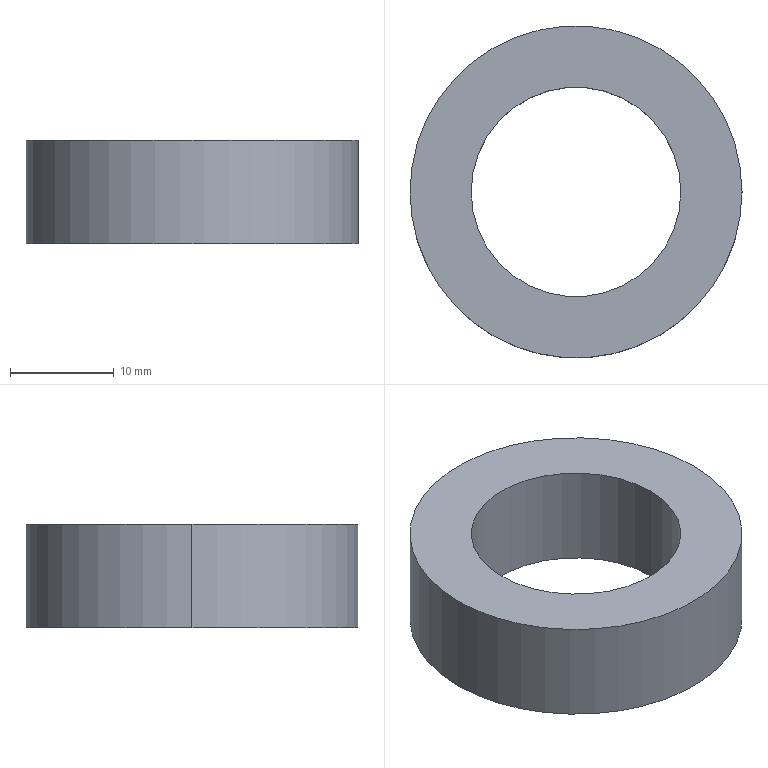Part | SolidWorks | features Extrusion 1 | 1 solid | 6 faces | box 32 x 32 x 10 mm | volume 4838 mm3 | cylinder 4 | plane 2 | commonest cylinder face diameters 20.2 x2 32 x2
STEP:
#1=CARTESIAN_POINT('',(-10.1,0.,-5.));
#2=VERTEX_POINT('',#1);
#3=CARTESIAN_POINT('',(10.1,0.,-5.));
#4=VERTEX_POINT('',#3);
#5=CARTESIAN_POINT('',(0.,0.,-5.));
#6=DIRECTION('',(0.,0.,1.));
#7=DIRECTION('',(1.,0.,0.));
#8=AXIS2_PLACEMENT_3D('',#5,#6,#7);
#9=CIRCLE('',#8,10.1);
#10=EDGE_CURVE('',#2,#4,#9,.T.);
#11=ORIENTED_EDGE('',*,*,#10,.F.);
#12=CARTESIAN_POINT('',(-10.1,0.,5.));
#13=VERTEX_POINT('',#12);
#14=CARTESIAN_POINT('',(-10.1,0.,-5.));
#15=DIRECTION('',(0.,0.,1.));
#16=VECTOR('',#15,1000.);
#17=LINE('',#14,#16);
#18=EDGE_CURVE('',#2,#13,#17,.T.);
#19=ORIENTED_EDGE('',*,*,#18,.T.);
#20=CARTESIAN_POINT('',(10.1,0.,5.));
#21=VERTEX_POINT('',#20);
#22=CARTESIAN_POINT('',(0.,0.,5.));
#23=DIRECTION('',(0.,0.,1.));
#24=DIRECTION('',(1.,0.,0.));
#25=AXIS2_PLACEMENT_3D('',#22,#23,#24);
#26=CIRCLE('',#25,10.1);
#27=EDGE_CURVE('',#13,#21,#26,.T.);
#28=ORIENTED_EDGE('',*,*,#27,.T.);
#29=CARTESIAN_POINT('',(10.1,0.,-5.));
#30=DIRECTION('',(0.,0.,1.));
#31=VECTOR('',#30,1000.);
#32=LINE('',#29,#31);
#33=EDGE_CURVE('',#4,#21,#32,.T.);
#34=ORIENTED_EDGE('',*,*,#33,.F.);
#35=EDGE_LOOP('',(#11,#19,#28,#34));
#36=FACE_OUTER_BOUND('',#35,.T.);
#37=CARTESIAN_POINT('',(0.,0.,-5.));
#38=DIRECTION('',(0.,0.,1.));
#39=DIRECTION('',(1.,0.,0.));
#40=AXIS2_PLACEMENT_3D('',#37,#38,#39);
#41=CYLINDRICAL_SURFACE('',#40,10.1);
#42=ADVANCED_FACE('',(#36),#41,.F.);
#43=CARTESIAN_POINT('',(16.,0.,-5.));
#44=VERTEX_POINT('',#43);
#45=CARTESIAN_POINT('',(-16.,0.,-5.));
#46=VERTEX_POINT('',#45);
#47=CARTESIAN_POINT('',(0.,0.,-5.));
#48=DIRECTION('',(0.,0.,1.));
#49=DIRECTION('',(1.,0.,0.));
#50=AXIS2_PLACEMENT_3D('',#47,#48,#49);
#51=CIRCLE('',#50,16.);
#52=EDGE_CURVE('',#44,#46,#51,.T.);
#53=ORIENTED_EDGE('',*,*,#52,.T.);
#54=CARTESIAN_POINT('',(-16.,0.,5.));
#55=VERTEX_POINT('',#54);
#56=CARTESIAN_POINT('',(-16.,0.,-5.));
#57=DIRECTION('',(0.,0.,1.));
#58=VECTOR('',#57,1000.);
#59=LINE('',#56,#58);
#60=EDGE_CURVE('',#46,#55,#59,.T.);
#61=ORIENTED_EDGE('',*,*,#60,.T.);
#62=CARTESIAN_POINT('',(16.,0.,5.));
#63=VERTEX_POINT('',#62);
#64=CARTESIAN_POINT('',(0.,0.,5.));
#65=DIRECTION('',(0.,0.,1.));
#66=DIRECTION('',(1.,0.,0.));
#67=AXIS2_PLACEMENT_3D('',#64,#65,#66);
#68=CIRCLE('',#67,16.);
#69=EDGE_CURVE('',#63,#55,#68,.T.);
#70=ORIENTED_EDGE('',*,*,#69,.F.);
#71=CARTESIAN_POINT('',(16.,0.,-5.));
#72=DIRECTION('',(0.,0.,1.));
#73=VECTOR('',#72,1000.);
#74=LINE('',#71,#73);
#75=EDGE_CURVE('',#44,#63,#74,.T.);
#76=ORIENTED_EDGE('',*,*,#75,.F.);
#77=EDGE_LOOP('',(#53,#61,#70,#76));
#78=FACE_OUTER_BOUND('',#77,.T.);
#79=CARTESIAN_POINT('',(0.,0.,-5.));
#80=DIRECTION('',(0.,0.,1.));
#81=DIRECTION('',(1.,0.,0.));
#82=AXIS2_PLACEMENT_3D('',#79,#80,#81);
#83=CYLINDRICAL_SURFACE('',#82,16.);
#84=ADVANCED_FACE('',(#78),#83,.T.);
#85=ORIENTED_EDGE('',*,*,#60,.F.);
#86=CARTESIAN_POINT('',(0.,0.,-5.));
#87=DIRECTION('',(0.,0.,1.));
#88=DIRECTION('',(1.,0.,0.));
#89=AXIS2_PLACEMENT_3D('',#86,#87,#88);
#90=CIRCLE('',#89,16.);
#91=EDGE_CURVE('',#46,#44,#90,.T.);
#92=ORIENTED_EDGE('',*,*,#91,.T.);
#93=ORIENTED_EDGE('',*,*,#75,.T.);
#94=CARTESIAN_POINT('',(0.,0.,5.));
#95=DIRECTION('',(0.,0.,1.));
#96=DIRECTION('',(1.,0.,0.));
#97=AXIS2_PLACEMENT_3D('',#94,#95,#96);
#98=CIRCLE('',#97,16.);
#99=EDGE_CURVE('',#55,#63,#98,.T.);
#100=ORIENTED_EDGE('',*,*,#99,.F.);
#101=EDGE_LOOP('',(#85,#92,#93,#100));
#102=FACE_OUTER_BOUND('',#101,.T.);
#103=CARTESIAN_POINT('',(0.,0.,-5.));
#104=DIRECTION('',(0.,0.,1.));
#105=DIRECTION('',(1.,0.,0.));
#106=AXIS2_PLACEMENT_3D('',#103,#104,#105);
#107=CYLINDRICAL_SURFACE('',#106,16.);
#108=ADVANCED_FACE('',(#102),#107,.T.);
#109=CARTESIAN_POINT('',(0.,0.,-5.));
#110=DIRECTION('',(0.,0.,1.));
#111=DIRECTION('',(1.,0.,0.));
#112=AXIS2_PLACEMENT_3D('',#109,#110,#111);
#113=CIRCLE('',#112,10.1);
#114=EDGE_CURVE('',#4,#2,#113,.T.);
#115=ORIENTED_EDGE('',*,*,#114,.T.);
#116=ORIENTED_EDGE('',*,*,#10,.T.);
#117=EDGE_LOOP('',(#115,#116));
#118=FACE_BOUND('',#117,.T.);
#119=ORIENTED_EDGE('',*,*,#52,.F.);
#120=ORIENTED_EDGE('',*,*,#91,.F.);
#121=EDGE_LOOP('',(#119,#120));
#122=FACE_OUTER_BOUND('',#121,.T.);
#123=CARTESIAN_POINT('',(0.,0.,-5.));
#124=DIRECTION('',(0.,0.,1.));
#125=DIRECTION('',(1.,0.,0.));
#126=AXIS2_PLACEMENT_3D('',#123,#124,#125);
#127=PLANE('',#126);
#128=ADVANCED_FACE('',(#118,#122),#127,.F.);
#129=CARTESIAN_POINT('',(0.,0.,5.));
#130=DIRECTION('',(0.,0.,1.));
#131=DIRECTION('',(1.,0.,0.));
#132=AXIS2_PLACEMENT_3D('',#129,#130,#131);
#133=CIRCLE('',#132,10.1);
#134=EDGE_CURVE('',#21,#13,#133,.T.);
#135=ORIENTED_EDGE('',*,*,#134,.F.);
#136=ORIENTED_EDGE('',*,*,#27,.F.);
#137=EDGE_LOOP('',(#135,#136));
#138=FACE_BOUND('',#137,.T.);
#139=ORIENTED_EDGE('',*,*,#69,.T.);
#140=ORIENTED_EDGE('',*,*,#99,.T.);
#141=EDGE_LOOP('',(#139,#140));
#142=FACE_OUTER_BOUND('',#141,.T.);
#143=CARTESIAN_POINT('',(0.,0.,5.));
#144=DIRECTION('',(0.,0.,1.));
#145=DIRECTION('',(1.,0.,0.));
#146=AXIS2_PLACEMENT_3D('',#143,#144,#145);
#147=PLANE('',#146);
#148=ADVANCED_FACE('',(#138,#142),#147,.T.);
#149=ORIENTED_EDGE('',*,*,#18,.F.);
#150=ORIENTED_EDGE('',*,*,#114,.F.);
#151=ORIENTED_EDGE('',*,*,#33,.T.);
#152=ORIENTED_EDGE('',*,*,#134,.T.);
#153=EDGE_LOOP('',(#149,#150,#151,#152));
#154=FACE_OUTER_BOUND('',#153,.T.);
#155=CARTESIAN_POINT('',(0.,0.,-5.));
#156=DIRECTION('',(0.,0.,1.));
#157=DIRECTION('',(1.,0.,0.));
#158=AXIS2_PLACEMENT_3D('',#155,#156,#157);
#159=CYLINDRICAL_SURFACE('',#158,10.1);
#160=ADVANCED_FACE('',(#154),#159,.F.);
#161=CLOSED_SHELL('',(#42,#84,#108,#128,#148,#160));
#162=MANIFOLD_SOLID_BREP('',#161);
#163=CARTESIAN_POINT('',(0.,0.,0.));
#164=DIRECTION('',(0.,0.,1.));
#165=DIRECTION('',(1.,0.,0.));
#166=AXIS2_PLACEMENT_3D('',#163,#164,#165);
#167=(LENGTH_UNIT()NAMED_UNIT(*)SI_UNIT(.MILLI.,.METRE.));
#168=UNCERTAINTY_MEASURE_WITH_UNIT(LENGTH_MEASURE(0.00001),#167,'','');
#169=(NAMED_UNIT(*)PLANE_ANGLE_UNIT()SI_UNIT($,.RADIAN.));
#170=(NAMED_UNIT(*)SI_UNIT($,.STERADIAN.)SOLID_ANGLE_UNIT());
#171=(GEOMETRIC_REPRESENTATION_CONTEXT(3)GLOBAL_UNCERTAINTY_ASSIGNED_CONTEXT((#168))GLOBAL_UNIT_ASSIGNED_CONTEXT((#167,#169,#170))REPRESENTATION_CONTEXT('',''));
#172=ADVANCED_BREP_SHAPE_REPRESENTATION('',(#162,#166),#171);